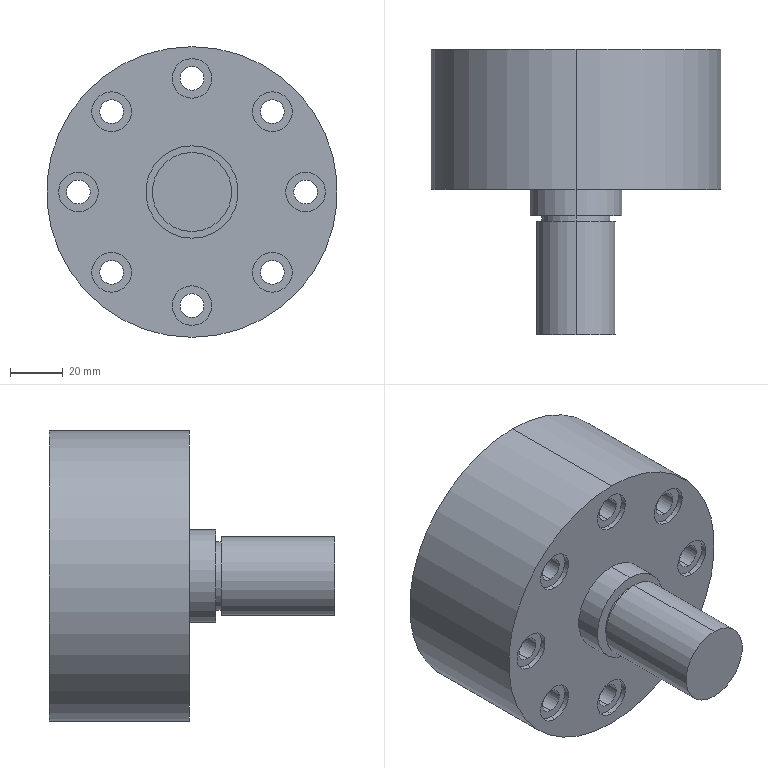Part | SolidWorks | features ICE 6, Revolution 1 | 1 solid | 56 faces | box 110 x 108 x 110 mm | volume 515028 mm3 | cylinder 42 | plane 14 | commonest cylinder face diameters 9 x16 15 x16 10 x2 26 x2 30 x2 35 x2